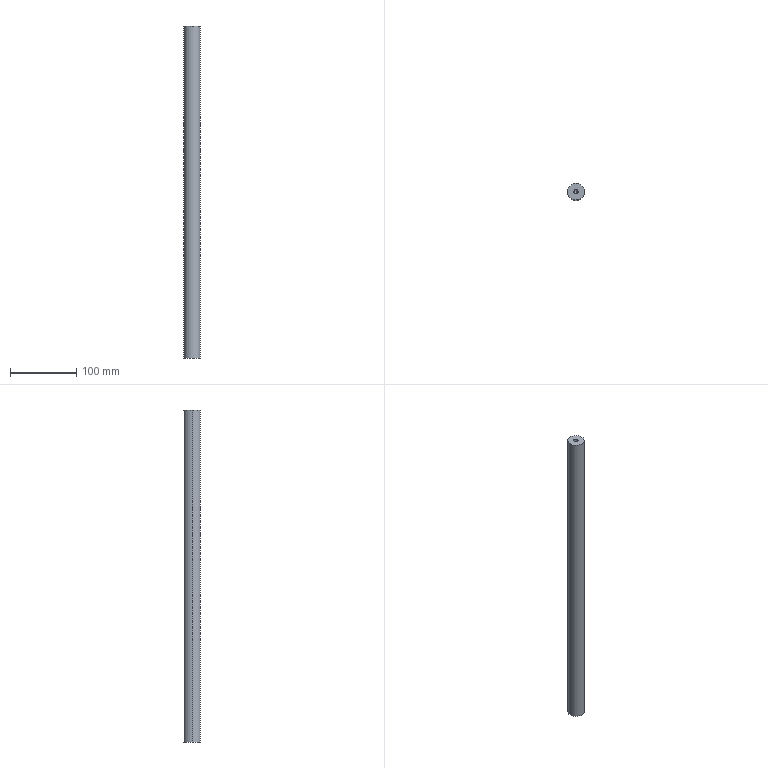Part | 1 solid | 8 faces | box 25 x 25 x 500 mm | volume 244686 mm3 | cylinder 4 | cone 2 | plane 2 | commonest cylinder face diameters 6.8 x2 25 x2
STEP:
#1=CARTESIAN_POINT('',(-3.4,0.,230.));
#2=VERTEX_POINT('',#1);
#3=CARTESIAN_POINT('',(3.4,0.,230.));
#4=VERTEX_POINT('',#3);
#5=CARTESIAN_POINT('',(0.,0.,230.));
#6=DIRECTION('',(0.,0.,1.));
#7=DIRECTION('',(1.,0.,0.));
#8=AXIS2_PLACEMENT_3D('',#5,#6,#7);
#9=CIRCLE('',#8,3.4);
#10=EDGE_CURVE('',#2,#4,#9,.T.);
#11=ORIENTED_EDGE('',*,*,#10,.F.);
#12=CARTESIAN_POINT('',(-3.4,0.,250.));
#13=VERTEX_POINT('',#12);
#14=CARTESIAN_POINT('',(-3.4,0.,250.));
#15=DIRECTION('',(0.,0.,1.));
#16=VECTOR('',#15,1000.);
#17=LINE('',#14,#16);
#18=EDGE_CURVE('',#2,#13,#17,.T.);
#19=ORIENTED_EDGE('',*,*,#18,.T.);
#20=CARTESIAN_POINT('',(3.4,0.,250.));
#21=VERTEX_POINT('',#20);
#22=CARTESIAN_POINT('',(0.,0.,250.));
#23=DIRECTION('',(0.,0.,1.));
#24=DIRECTION('',(1.,0.,0.));
#25=AXIS2_PLACEMENT_3D('',#22,#23,#24);
#26=CIRCLE('',#25,3.4);
#27=EDGE_CURVE('',#13,#21,#26,.T.);
#28=ORIENTED_EDGE('',*,*,#27,.T.);
#29=CARTESIAN_POINT('',(3.4,0.,250.));
#30=DIRECTION('',(0.,0.,1.));
#31=VECTOR('',#30,1000.);
#32=LINE('',#29,#31);
#33=EDGE_CURVE('',#4,#21,#32,.T.);
#34=ORIENTED_EDGE('',*,*,#33,.F.);
#35=EDGE_LOOP('',(#11,#19,#28,#34));
#36=FACE_OUTER_BOUND('',#35,.T.);
#37=CARTESIAN_POINT('',(0.,0.,250.));
#38=DIRECTION('',(0.,0.,1.));
#39=DIRECTION('',(1.,0.,0.));
#40=AXIS2_PLACEMENT_3D('',#37,#38,#39);
#41=CYLINDRICAL_SURFACE('',#40,3.4);
#42=ADVANCED_FACE('',(#36),#41,.F.);
#43=CARTESIAN_POINT('',(0.,0.,227.957));
#44=VERTEX_POINT('',#43);
#45=CARTESIAN_POINT('',(3.4,0.,230.));
#46=DIRECTION('',(0.8572,0.,0.515));
#47=VECTOR('',#46,1000.);
#48=LINE('',#45,#47);
#49=EDGE_CURVE('',#44,#4,#48,.T.);
#50=ORIENTED_EDGE('',*,*,#49,.F.);
#51=CARTESIAN_POINT('',(-3.4,0.,230.));
#52=DIRECTION('',(-0.8572,0.,0.515));
#53=VECTOR('',#52,1000.);
#54=LINE('',#51,#53);
#55=EDGE_CURVE('',#44,#2,#54,.T.);
#56=ORIENTED_EDGE('',*,*,#55,.T.);
#57=ORIENTED_EDGE('',*,*,#10,.T.);
#58=EDGE_LOOP('',(#50,#56,#57));
#59=FACE_OUTER_BOUND('',#58,.T.);
#60=CARTESIAN_POINT('',(0.,0.,230.));
#61=DIRECTION('',(0.,0.,1.));
#62=DIRECTION('',(1.,0.,0.));
#63=AXIS2_PLACEMENT_3D('',#60,#61,#62);
#64=CONICAL_SURFACE('',#63,3.4,1.03);
#65=ADVANCED_FACE('',(#59),#64,.F.);
#66=CARTESIAN_POINT('',(12.5,0.,250.));
#67=VERTEX_POINT('',#66);
#68=CARTESIAN_POINT('',(-12.5,0.,250.));
#69=VERTEX_POINT('',#68);
#70=CARTESIAN_POINT('',(0.,0.,250.));
#71=DIRECTION('',(0.,0.,1.));
#72=DIRECTION('',(1.,0.,0.));
#73=AXIS2_PLACEMENT_3D('',#70,#71,#72);
#74=CIRCLE('',#73,12.5);
#75=EDGE_CURVE('',#67,#69,#74,.T.);
#76=ORIENTED_EDGE('',*,*,#75,.F.);
#77=CARTESIAN_POINT('',(12.5,0.,-250.));
#78=VERTEX_POINT('',#77);
#79=CARTESIAN_POINT('',(12.5,0.,250.));
#80=DIRECTION('',(0.,0.,-1.));
#81=VECTOR('',#80,1000.);
#82=LINE('',#79,#81);
#83=EDGE_CURVE('',#67,#78,#82,.T.);
#84=ORIENTED_EDGE('',*,*,#83,.T.);
#85=CARTESIAN_POINT('',(-12.5,0.,-250.));
#86=VERTEX_POINT('',#85);
#87=CARTESIAN_POINT('',(0.,0.,-250.));
#88=DIRECTION('',(0.,0.,1.));
#89=DIRECTION('',(1.,0.,0.));
#90=AXIS2_PLACEMENT_3D('',#87,#88,#89);
#91=CIRCLE('',#90,12.5);
#92=EDGE_CURVE('',#78,#86,#91,.T.);
#93=ORIENTED_EDGE('',*,*,#92,.T.);
#94=CARTESIAN_POINT('',(-12.5,0.,250.));
#95=DIRECTION('',(0.,0.,-1.));
#96=VECTOR('',#95,1000.);
#97=LINE('',#94,#96);
#98=EDGE_CURVE('',#69,#86,#97,.T.);
#99=ORIENTED_EDGE('',*,*,#98,.F.);
#100=EDGE_LOOP('',(#76,#84,#93,#99));
#101=FACE_OUTER_BOUND('',#100,.T.);
#102=CARTESIAN_POINT('',(0.,0.,250.));
#103=DIRECTION('',(0.,0.,-1.));
#104=DIRECTION('',(-1.,0.,0.));
#105=AXIS2_PLACEMENT_3D('',#102,#103,#104);
#106=CYLINDRICAL_SURFACE('',#105,12.5);
#107=ADVANCED_FACE('',(#101),#106,.T.);
#108=ORIENTED_EDGE('',*,*,#83,.F.);
#109=CARTESIAN_POINT('',(0.,0.,250.));
#110=DIRECTION('',(0.,0.,1.));
#111=DIRECTION('',(1.,0.,0.));
#112=AXIS2_PLACEMENT_3D('',#109,#110,#111);
#113=CIRCLE('',#112,12.5);
#114=EDGE_CURVE('',#69,#67,#113,.T.);
#115=ORIENTED_EDGE('',*,*,#114,.F.);
#116=ORIENTED_EDGE('',*,*,#98,.T.);
#117=CARTESIAN_POINT('',(0.,0.,-250.));
#118=DIRECTION('',(0.,0.,1.));
#119=DIRECTION('',(1.,0.,0.));
#120=AXIS2_PLACEMENT_3D('',#117,#118,#119);
#121=CIRCLE('',#120,12.5);
#122=EDGE_CURVE('',#86,#78,#121,.T.);
#123=ORIENTED_EDGE('',*,*,#122,.T.);
#124=EDGE_LOOP('',(#108,#115,#116,#123));
#125=FACE_OUTER_BOUND('',#124,.T.);
#126=CARTESIAN_POINT('',(0.,0.,250.));
#127=DIRECTION('',(0.,0.,-1.));
#128=DIRECTION('',(-1.,0.,0.));
#129=AXIS2_PLACEMENT_3D('',#126,#127,#128);
#130=CYLINDRICAL_SURFACE('',#129,12.5);
#131=ADVANCED_FACE('',(#125),#130,.T.);
#132=CARTESIAN_POINT('',(0.,0.,250.));
#133=DIRECTION('',(0.,0.,1.));
#134=DIRECTION('',(1.,0.,0.));
#135=AXIS2_PLACEMENT_3D('',#132,#133,#134);
#136=CIRCLE('',#135,3.4);
#137=EDGE_CURVE('',#21,#13,#136,.T.);
#138=ORIENTED_EDGE('',*,*,#137,.F.);
#139=ORIENTED_EDGE('',*,*,#27,.F.);
#140=EDGE_LOOP('',(#138,#139));
#141=FACE_BOUND('',#140,.T.);
#142=ORIENTED_EDGE('',*,*,#114,.T.);
#143=ORIENTED_EDGE('',*,*,#75,.T.);
#144=EDGE_LOOP('',(#142,#143));
#145=FACE_OUTER_BOUND('',#144,.T.);
#146=CARTESIAN_POINT('',(0.,0.,250.));
#147=DIRECTION('',(0.,0.,1.));
#148=DIRECTION('',(1.,0.,0.));
#149=AXIS2_PLACEMENT_3D('',#146,#147,#148);
#150=PLANE('',#149);
#151=ADVANCED_FACE('',(#141,#145),#150,.T.);
#152=ORIENTED_EDGE('',*,*,#122,.F.);
#153=ORIENTED_EDGE('',*,*,#92,.F.);
#154=EDGE_LOOP('',(#152,#153));
#155=FACE_OUTER_BOUND('',#154,.T.);
#156=CARTESIAN_POINT('',(0.,0.,-250.));
#157=DIRECTION('',(0.,0.,1.));
#158=DIRECTION('',(1.,0.,0.));
#159=AXIS2_PLACEMENT_3D('',#156,#157,#158);
#160=PLANE('',#159);
#161=ADVANCED_FACE('',(#155),#160,.F.);
#162=ORIENTED_EDGE('',*,*,#55,.F.);
#163=ORIENTED_EDGE('',*,*,#49,.T.);
#164=CARTESIAN_POINT('',(0.,0.,230.));
#165=DIRECTION('',(0.,0.,1.));
#166=DIRECTION('',(1.,0.,0.));
#167=AXIS2_PLACEMENT_3D('',#164,#165,#166);
#168=CIRCLE('',#167,3.4);
#169=EDGE_CURVE('',#4,#2,#168,.T.);
#170=ORIENTED_EDGE('',*,*,#169,.T.);
#171=EDGE_LOOP('',(#162,#163,#170));
#172=FACE_OUTER_BOUND('',#171,.T.);
#173=CARTESIAN_POINT('',(0.,0.,230.));
#174=DIRECTION('',(0.,0.,1.));
#175=DIRECTION('',(1.,0.,0.));
#176=AXIS2_PLACEMENT_3D('',#173,#174,#175);
#177=CONICAL_SURFACE('',#176,3.4,1.03);
#178=ADVANCED_FACE('',(#172),#177,.F.);
#179=ORIENTED_EDGE('',*,*,#18,.F.);
#180=ORIENTED_EDGE('',*,*,#169,.F.);
#181=ORIENTED_EDGE('',*,*,#33,.T.);
#182=ORIENTED_EDGE('',*,*,#137,.T.);
#183=EDGE_LOOP('',(#179,#180,#181,#182));
#184=FACE_OUTER_BOUND('',#183,.T.);
#185=CARTESIAN_POINT('',(0.,0.,250.));
#186=DIRECTION('',(0.,0.,1.));
#187=DIRECTION('',(1.,0.,0.));
#188=AXIS2_PLACEMENT_3D('',#185,#186,#187);
#189=CYLINDRICAL_SURFACE('',#188,3.4);
#190=ADVANCED_FACE('',(#184),#189,.F.);
#191=CLOSED_SHELL('',(#42,#65,#107,#131,#151,#161,#178,#190));
#192=MANIFOLD_SOLID_BREP('',#191);
#193=CARTESIAN_POINT('',(0.,0.,0.));
#194=DIRECTION('',(0.,0.,1.));
#195=DIRECTION('',(1.,0.,0.));
#196=AXIS2_PLACEMENT_3D('',#193,#194,#195);
#197=(LENGTH_UNIT()NAMED_UNIT(*)SI_UNIT(.MILLI.,.METRE.));
#198=UNCERTAINTY_MEASURE_WITH_UNIT(LENGTH_MEASURE(0.00001),#197,'','');
#199=(NAMED_UNIT(*)PLANE_ANGLE_UNIT()SI_UNIT($,.RADIAN.));
#200=(NAMED_UNIT(*)SI_UNIT($,.STERADIAN.)SOLID_ANGLE_UNIT());
#201=(GEOMETRIC_REPRESENTATION_CONTEXT(3)GLOBAL_UNCERTAINTY_ASSIGNED_CONTEXT((#198))GLOBAL_UNIT_ASSIGNED_CONTEXT((#197,#199,#200))REPRESENTATION_CONTEXT('',''));
#202=ADVANCED_BREP_SHAPE_REPRESENTATION('',(#192,#196),#201);